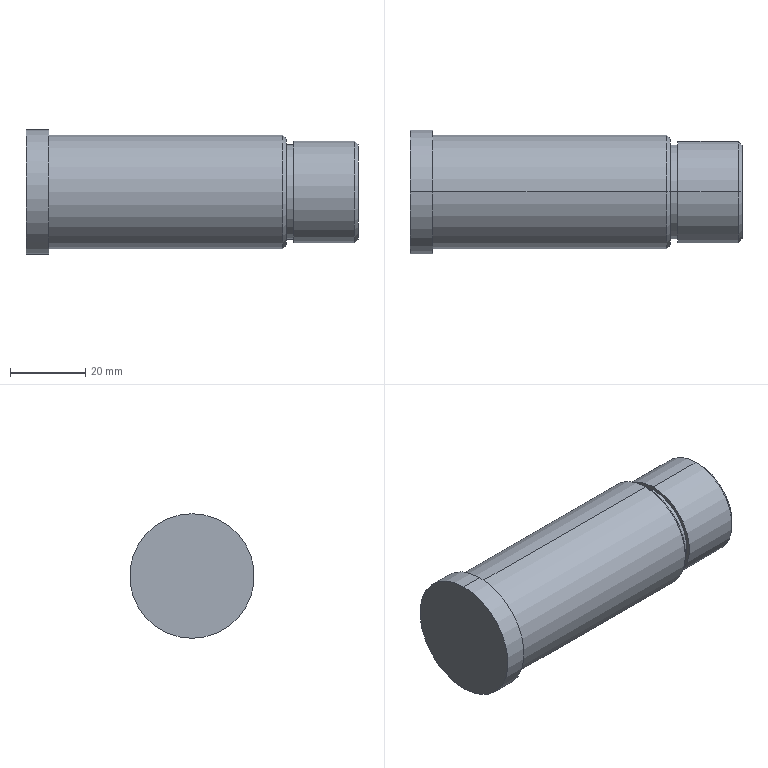Part | SolidWorks | features Chamfer 1, Revolution 1 | 1 solid | 17 faces | box 88 x 33 x 33 mm | volume 60292 mm3 | cylinder 8 | plane 5 | cone 4 | commonest cylinder face diameters 25 x2 27 x2 30 x2 33 x2
STEP:
#1=CARTESIAN_POINT('',(69.,0.,-14.));
#2=VERTEX_POINT('',#1);
#3=CARTESIAN_POINT('',(69.,0.,14.));
#4=VERTEX_POINT('',#3);
#5=CARTESIAN_POINT('',(69.,0.,0.));
#6=DIRECTION('',(1.,0.,0.));
#7=DIRECTION('',(0.,0.,1.));
#8=AXIS2_PLACEMENT_3D('',#5,#6,#7);
#9=CIRCLE('',#8,14.);
#10=EDGE_CURVE('',#2,#4,#9,.T.);
#11=ORIENTED_EDGE('',*,*,#10,.F.);
#12=CARTESIAN_POINT('',(68.,0.,-15.));
#13=VERTEX_POINT('',#12);
#14=CARTESIAN_POINT('',(68.,0.,-15.));
#15=DIRECTION('',(-0.7071,0.,-0.7071));
#16=VECTOR('',#15,1000.);
#17=LINE('',#14,#16);
#18=EDGE_CURVE('',#2,#13,#17,.T.);
#19=ORIENTED_EDGE('',*,*,#18,.T.);
#20=CARTESIAN_POINT('',(68.,0.,15.));
#21=VERTEX_POINT('',#20);
#22=CARTESIAN_POINT('',(68.,0.,0.));
#23=DIRECTION('',(-1.,0.,0.));
#24=DIRECTION('',(0.,0.,1.));
#25=AXIS2_PLACEMENT_3D('',#22,#23,#24);
#26=CIRCLE('',#25,15.);
#27=EDGE_CURVE('',#21,#13,#26,.T.);
#28=ORIENTED_EDGE('',*,*,#27,.F.);
#29=CARTESIAN_POINT('',(68.,0.,15.));
#30=DIRECTION('',(-0.7071,0.,0.7071));
#31=VECTOR('',#30,1000.);
#32=LINE('',#29,#31);
#33=EDGE_CURVE('',#4,#21,#32,.T.);
#34=ORIENTED_EDGE('',*,*,#33,.F.);
#35=EDGE_LOOP('',(#11,#19,#28,#34));
#36=FACE_OUTER_BOUND('',#35,.T.);
#37=CARTESIAN_POINT('',(68.,0.,0.));
#38=DIRECTION('',(-1.,0.,0.));
#39=DIRECTION('',(0.,0.,1.));
#40=AXIS2_PLACEMENT_3D('',#37,#38,#39);
#41=CONICAL_SURFACE('',#40,15.,0.7854);
#42=ADVANCED_FACE('',(#36),#41,.T.);
#43=CARTESIAN_POINT('',(88.,0.,-12.5));
#44=VERTEX_POINT('',#43);
#45=CARTESIAN_POINT('',(88.,0.,12.5));
#46=VERTEX_POINT('',#45);
#47=CARTESIAN_POINT('',(88.,0.,0.));
#48=DIRECTION('',(1.,0.,0.));
#49=DIRECTION('',(0.,0.,1.));
#50=AXIS2_PLACEMENT_3D('',#47,#48,#49);
#51=CIRCLE('',#50,12.5);
#52=EDGE_CURVE('',#44,#46,#51,.T.);
#53=ORIENTED_EDGE('',*,*,#52,.F.);
#54=CARTESIAN_POINT('',(87.,0.,-13.5));
#55=VERTEX_POINT('',#54);
#56=CARTESIAN_POINT('',(87.,0.,-13.5));
#57=DIRECTION('',(-0.7071,0.,-0.7071));
#58=VECTOR('',#57,1000.);
#59=LINE('',#56,#58);
#60=EDGE_CURVE('',#44,#55,#59,.T.);
#61=ORIENTED_EDGE('',*,*,#60,.T.);
#62=CARTESIAN_POINT('',(87.,0.,13.5));
#63=VERTEX_POINT('',#62);
#64=CARTESIAN_POINT('',(87.,0.,0.));
#65=DIRECTION('',(-1.,0.,0.));
#66=DIRECTION('',(0.,0.,1.));
#67=AXIS2_PLACEMENT_3D('',#64,#65,#66);
#68=CIRCLE('',#67,13.5);
#69=EDGE_CURVE('',#63,#55,#68,.T.);
#70=ORIENTED_EDGE('',*,*,#69,.F.);
#71=CARTESIAN_POINT('',(87.,0.,13.5));
#72=DIRECTION('',(-0.7071,0.,0.7071));
#73=VECTOR('',#72,1000.);
#74=LINE('',#71,#73);
#75=EDGE_CURVE('',#46,#63,#74,.T.);
#76=ORIENTED_EDGE('',*,*,#75,.F.);
#77=EDGE_LOOP('',(#53,#61,#70,#76));
#78=FACE_OUTER_BOUND('',#77,.T.);
#79=CARTESIAN_POINT('',(87.,0.,0.));
#80=DIRECTION('',(-1.,0.,0.));
#81=DIRECTION('',(0.,0.,1.));
#82=AXIS2_PLACEMENT_3D('',#79,#80,#81);
#83=CONICAL_SURFACE('',#82,13.5,0.7854);
#84=ADVANCED_FACE('',(#78),#83,.T.);
#85=ORIENTED_EDGE('',*,*,#69,.T.);
#86=CARTESIAN_POINT('',(71.,0.,-13.5));
#87=VERTEX_POINT('',#86);
#88=CARTESIAN_POINT('',(0.,0.,-13.5));
#89=DIRECTION('',(-1.,0.,0.));
#90=VECTOR('',#89,1000.);
#91=LINE('',#88,#90);
#92=EDGE_CURVE('',#55,#87,#91,.T.);
#93=ORIENTED_EDGE('',*,*,#92,.T.);
#94=CARTESIAN_POINT('',(71.,0.,13.5));
#95=VERTEX_POINT('',#94);
#96=CARTESIAN_POINT('',(71.,0.,0.));
#97=DIRECTION('',(-1.,0.,0.));
#98=DIRECTION('',(0.,0.,1.));
#99=AXIS2_PLACEMENT_3D('',#96,#97,#98);
#100=CIRCLE('',#99,13.5);
#101=EDGE_CURVE('',#95,#87,#100,.T.);
#102=ORIENTED_EDGE('',*,*,#101,.F.);
#103=CARTESIAN_POINT('',(0.,0.,13.5));
#104=DIRECTION('',(-1.,0.,0.));
#105=VECTOR('',#104,1000.);
#106=LINE('',#103,#105);
#107=EDGE_CURVE('',#63,#95,#106,.T.);
#108=ORIENTED_EDGE('',*,*,#107,.F.);
#109=EDGE_LOOP('',(#85,#93,#102,#108));
#110=FACE_OUTER_BOUND('',#109,.T.);
#111=CARTESIAN_POINT('',(0.,0.,0.));
#112=DIRECTION('',(-1.,0.,0.));
#113=DIRECTION('',(0.,0.,1.));
#114=AXIS2_PLACEMENT_3D('',#111,#112,#113);
#115=CYLINDRICAL_SURFACE('',#114,13.5);
#116=ADVANCED_FACE('',(#110),#115,.T.);
#117=CARTESIAN_POINT('',(71.,0.,12.5));
#118=VERTEX_POINT('',#117);
#119=CARTESIAN_POINT('',(71.,0.,-12.5));
#120=VERTEX_POINT('',#119);
#121=CARTESIAN_POINT('',(71.,0.,0.));
#122=DIRECTION('',(-1.,0.,0.));
#123=DIRECTION('',(0.,0.,1.));
#124=AXIS2_PLACEMENT_3D('',#121,#122,#123);
#125=CIRCLE('',#124,12.5);
#126=EDGE_CURVE('',#118,#120,#125,.T.);
#127=ORIENTED_EDGE('',*,*,#126,.T.);
#128=CARTESIAN_POINT('',(69.,0.,-12.5));
#129=VERTEX_POINT('',#128);
#130=CARTESIAN_POINT('',(0.,0.,-12.5));
#131=DIRECTION('',(-1.,0.,0.));
#132=VECTOR('',#131,1000.);
#133=LINE('',#130,#132);
#134=EDGE_CURVE('',#120,#129,#133,.T.);
#135=ORIENTED_EDGE('',*,*,#134,.T.);
#136=CARTESIAN_POINT('',(69.,0.,12.5));
#137=VERTEX_POINT('',#136);
#138=CARTESIAN_POINT('',(69.,0.,0.));
#139=DIRECTION('',(-1.,0.,0.));
#140=DIRECTION('',(0.,0.,1.));
#141=AXIS2_PLACEMENT_3D('',#138,#139,#140);
#142=CIRCLE('',#141,12.5);
#143=EDGE_CURVE('',#137,#129,#142,.T.);
#144=ORIENTED_EDGE('',*,*,#143,.F.);
#145=CARTESIAN_POINT('',(0.,0.,12.5));
#146=DIRECTION('',(-1.,0.,0.));
#147=VECTOR('',#146,1000.);
#148=LINE('',#145,#147);
#149=EDGE_CURVE('',#118,#137,#148,.T.);
#150=ORIENTED_EDGE('',*,*,#149,.F.);
#151=EDGE_LOOP('',(#127,#135,#144,#150));
#152=FACE_OUTER_BOUND('',#151,.T.);
#153=CARTESIAN_POINT('',(0.,0.,0.));
#154=DIRECTION('',(-1.,0.,0.));
#155=DIRECTION('',(0.,0.,1.));
#156=AXIS2_PLACEMENT_3D('',#153,#154,#155);
#157=CYLINDRICAL_SURFACE('',#156,12.5);
#158=ADVANCED_FACE('',(#152),#157,.T.);
#159=ORIENTED_EDGE('',*,*,#27,.T.);
#160=CARTESIAN_POINT('',(6.,0.,-15.));
#161=VERTEX_POINT('',#160);
#162=CARTESIAN_POINT('',(0.,0.,-15.));
#163=DIRECTION('',(-1.,0.,0.));
#164=VECTOR('',#163,1000.);
#165=LINE('',#162,#164);
#166=EDGE_CURVE('',#13,#161,#165,.T.);
#167=ORIENTED_EDGE('',*,*,#166,.T.);
#168=CARTESIAN_POINT('',(6.,0.,15.));
#169=VERTEX_POINT('',#168);
#170=CARTESIAN_POINT('',(6.,0.,0.));
#171=DIRECTION('',(-1.,0.,0.));
#172=DIRECTION('',(0.,0.,1.));
#173=AXIS2_PLACEMENT_3D('',#170,#171,#172);
#174=CIRCLE('',#173,15.);
#175=EDGE_CURVE('',#169,#161,#174,.T.);
#176=ORIENTED_EDGE('',*,*,#175,.F.);
#177=CARTESIAN_POINT('',(0.,0.,15.));
#178=DIRECTION('',(-1.,0.,0.));
#179=VECTOR('',#178,1000.);
#180=LINE('',#177,#179);
#181=EDGE_CURVE('',#21,#169,#180,.T.);
#182=ORIENTED_EDGE('',*,*,#181,.F.);
#183=EDGE_LOOP('',(#159,#167,#176,#182));
#184=FACE_OUTER_BOUND('',#183,.T.);
#185=CARTESIAN_POINT('',(0.,0.,0.));
#186=DIRECTION('',(-1.,0.,0.));
#187=DIRECTION('',(0.,0.,1.));
#188=AXIS2_PLACEMENT_3D('',#185,#186,#187);
#189=CYLINDRICAL_SURFACE('',#188,15.);
#190=ADVANCED_FACE('',(#184),#189,.T.);
#191=CARTESIAN_POINT('',(6.,0.,16.5));
#192=VERTEX_POINT('',#191);
#193=CARTESIAN_POINT('',(6.,0.,-16.5));
#194=VERTEX_POINT('',#193);
#195=CARTESIAN_POINT('',(6.,0.,0.));
#196=DIRECTION('',(-1.,0.,0.));
#197=DIRECTION('',(0.,0.,1.));
#198=AXIS2_PLACEMENT_3D('',#195,#196,#197);
#199=CIRCLE('',#198,16.5);
#200=EDGE_CURVE('',#192,#194,#199,.T.);
#201=ORIENTED_EDGE('',*,*,#200,.T.);
#202=CARTESIAN_POINT('',(0.,0.,-16.5));
#203=VERTEX_POINT('',#202);
#204=CARTESIAN_POINT('',(0.,0.,-16.5));
#205=DIRECTION('',(-1.,0.,0.));
#206=VECTOR('',#205,1000.);
#207=LINE('',#204,#206);
#208=EDGE_CURVE('',#194,#203,#207,.T.);
#209=ORIENTED_EDGE('',*,*,#208,.T.);
#210=CARTESIAN_POINT('',(0.,0.,16.5));
#211=VERTEX_POINT('',#210);
#212=CARTESIAN_POINT('',(0.,0.,0.));
#213=DIRECTION('',(-1.,0.,0.));
#214=DIRECTION('',(0.,0.,1.));
#215=AXIS2_PLACEMENT_3D('',#212,#213,#214);
#216=CIRCLE('',#215,16.5);
#217=EDGE_CURVE('',#211,#203,#216,.T.);
#218=ORIENTED_EDGE('',*,*,#217,.F.);
#219=CARTESIAN_POINT('',(0.,0.,16.5));
#220=DIRECTION('',(-1.,0.,0.));
#221=VECTOR('',#220,1000.);
#222=LINE('',#219,#221);
#223=EDGE_CURVE('',#192,#211,#222,.T.);
#224=ORIENTED_EDGE('',*,*,#223,.F.);
#225=EDGE_LOOP('',(#201,#209,#218,#224));
#226=FACE_OUTER_BOUND('',#225,.T.);
#227=CARTESIAN_POINT('',(0.,0.,0.));
#228=DIRECTION('',(-1.,0.,0.));
#229=DIRECTION('',(0.,0.,1.));
#230=AXIS2_PLACEMENT_3D('',#227,#228,#229);
#231=CYLINDRICAL_SURFACE('',#230,16.5);
#232=ADVANCED_FACE('',(#226),#231,.T.);
#233=ORIENTED_EDGE('',*,*,#217,.T.);
#234=CARTESIAN_POINT('',(0.,0.,0.));
#235=DIRECTION('',(-1.,0.,0.));
#236=DIRECTION('',(0.,0.,1.));
#237=AXIS2_PLACEMENT_3D('',#234,#235,#236);
#238=CIRCLE('',#237,16.5);
#239=EDGE_CURVE('',#203,#211,#238,.T.);
#240=ORIENTED_EDGE('',*,*,#239,.T.);
#241=EDGE_LOOP('',(#233,#240));
#242=FACE_OUTER_BOUND('',#241,.T.);
#243=CARTESIAN_POINT('',(0.,0.,0.));
#244=DIRECTION('',(1.,0.,0.));
#245=DIRECTION('',(0.,0.,-1.));
#246=AXIS2_PLACEMENT_3D('',#243,#244,#245);
#247=PLANE('',#246);
#248=ADVANCED_FACE('',(#242),#247,.F.);
#249=ORIENTED_EDGE('',*,*,#208,.F.);
#250=CARTESIAN_POINT('',(6.,0.,0.));
#251=DIRECTION('',(-1.,0.,0.));
#252=DIRECTION('',(0.,0.,1.));
#253=AXIS2_PLACEMENT_3D('',#250,#251,#252);
#254=CIRCLE('',#253,16.5);
#255=EDGE_CURVE('',#194,#192,#254,.T.);
#256=ORIENTED_EDGE('',*,*,#255,.T.);
#257=ORIENTED_EDGE('',*,*,#223,.T.);
#258=ORIENTED_EDGE('',*,*,#239,.F.);
#259=EDGE_LOOP('',(#249,#256,#257,#258));
#260=FACE_OUTER_BOUND('',#259,.T.);
#261=CARTESIAN_POINT('',(0.,0.,0.));
#262=DIRECTION('',(-1.,0.,0.));
#263=DIRECTION('',(0.,0.,1.));
#264=AXIS2_PLACEMENT_3D('',#261,#262,#263);
#265=CYLINDRICAL_SURFACE('',#264,16.5);
#266=ADVANCED_FACE('',(#260),#265,.T.);
#267=ORIENTED_EDGE('',*,*,#200,.F.);
#268=ORIENTED_EDGE('',*,*,#255,.F.);
#269=EDGE_LOOP('',(#267,#268));
#270=FACE_OUTER_BOUND('',#269,.T.);
#271=ORIENTED_EDGE('',*,*,#175,.T.);
#272=CARTESIAN_POINT('',(6.,0.,0.));
#273=DIRECTION('',(-1.,0.,0.));
#274=DIRECTION('',(0.,0.,1.));
#275=AXIS2_PLACEMENT_3D('',#272,#273,#274);
#276=CIRCLE('',#275,15.);
#277=EDGE_CURVE('',#161,#169,#276,.T.);
#278=ORIENTED_EDGE('',*,*,#277,.T.);
#279=EDGE_LOOP('',(#271,#278));
#280=FACE_BOUND('',#279,.T.);
#281=CARTESIAN_POINT('',(6.,16.5,0.));
#282=DIRECTION('',(-1.,0.,0.));
#283=DIRECTION('',(0.,0.,1.));
#284=AXIS2_PLACEMENT_3D('',#281,#282,#283);
#285=PLANE('',#284);
#286=ADVANCED_FACE('',(#270,#280),#285,.F.);
#287=ORIENTED_EDGE('',*,*,#166,.F.);
#288=CARTESIAN_POINT('',(68.,0.,0.));
#289=DIRECTION('',(-1.,0.,0.));
#290=DIRECTION('',(0.,0.,1.));
#291=AXIS2_PLACEMENT_3D('',#288,#289,#290);
#292=CIRCLE('',#291,15.);
#293=EDGE_CURVE('',#13,#21,#292,.T.);
#294=ORIENTED_EDGE('',*,*,#293,.T.);
#295=ORIENTED_EDGE('',*,*,#181,.T.);
#296=ORIENTED_EDGE('',*,*,#277,.F.);
#297=EDGE_LOOP('',(#287,#294,#295,#296));
#298=FACE_OUTER_BOUND('',#297,.T.);
#299=CARTESIAN_POINT('',(0.,0.,0.));
#300=DIRECTION('',(-1.,0.,0.));
#301=DIRECTION('',(0.,0.,1.));
#302=AXIS2_PLACEMENT_3D('',#299,#300,#301);
#303=CYLINDRICAL_SURFACE('',#302,15.);
#304=ADVANCED_FACE('',(#298),#303,.T.);
#305=CARTESIAN_POINT('',(69.,0.,0.));
#306=DIRECTION('',(1.,0.,0.));
#307=DIRECTION('',(0.,0.,1.));
#308=AXIS2_PLACEMENT_3D('',#305,#306,#307);
#309=CIRCLE('',#308,14.);
#310=EDGE_CURVE('',#4,#2,#309,.T.);
#311=ORIENTED_EDGE('',*,*,#310,.T.);
#312=ORIENTED_EDGE('',*,*,#10,.T.);
#313=EDGE_LOOP('',(#311,#312));
#314=FACE_OUTER_BOUND('',#313,.T.);
#315=ORIENTED_EDGE('',*,*,#143,.T.);
#316=CARTESIAN_POINT('',(69.,0.,0.));
#317=DIRECTION('',(-1.,0.,0.));
#318=DIRECTION('',(0.,0.,1.));
#319=AXIS2_PLACEMENT_3D('',#316,#317,#318);
#320=CIRCLE('',#319,12.5);
#321=EDGE_CURVE('',#129,#137,#320,.T.);
#322=ORIENTED_EDGE('',*,*,#321,.T.);
#323=EDGE_LOOP('',(#315,#322));
#324=FACE_BOUND('',#323,.T.);
#325=CARTESIAN_POINT('',(69.,15.,0.));
#326=DIRECTION('',(-1.,0.,0.));
#327=DIRECTION('',(0.,0.,1.));
#328=AXIS2_PLACEMENT_3D('',#325,#326,#327);
#329=PLANE('',#328);
#330=ADVANCED_FACE('',(#314,#324),#329,.F.);
#331=ORIENTED_EDGE('',*,*,#134,.F.);
#332=CARTESIAN_POINT('',(71.,0.,0.));
#333=DIRECTION('',(-1.,0.,0.));
#334=DIRECTION('',(0.,0.,1.));
#335=AXIS2_PLACEMENT_3D('',#332,#333,#334);
#336=CIRCLE('',#335,12.5);
#337=EDGE_CURVE('',#120,#118,#336,.T.);
#338=ORIENTED_EDGE('',*,*,#337,.T.);
#339=ORIENTED_EDGE('',*,*,#149,.T.);
#340=ORIENTED_EDGE('',*,*,#321,.F.);
#341=EDGE_LOOP('',(#331,#338,#339,#340));
#342=FACE_OUTER_BOUND('',#341,.T.);
#343=CARTESIAN_POINT('',(0.,0.,0.));
#344=DIRECTION('',(-1.,0.,0.));
#345=DIRECTION('',(0.,0.,1.));
#346=AXIS2_PLACEMENT_3D('',#343,#344,#345);
#347=CYLINDRICAL_SURFACE('',#346,12.5);
#348=ADVANCED_FACE('',(#342),#347,.T.);
#349=ORIENTED_EDGE('',*,*,#126,.F.);
#350=ORIENTED_EDGE('',*,*,#337,.F.);
#351=EDGE_LOOP('',(#349,#350));
#352=FACE_BOUND('',#351,.T.);
#353=ORIENTED_EDGE('',*,*,#101,.T.);
#354=CARTESIAN_POINT('',(71.,0.,0.));
#355=DIRECTION('',(-1.,0.,0.));
#356=DIRECTION('',(0.,0.,1.));
#357=AXIS2_PLACEMENT_3D('',#354,#355,#356);
#358=CIRCLE('',#357,13.5);
#359=EDGE_CURVE('',#87,#95,#358,.T.);
#360=ORIENTED_EDGE('',*,*,#359,.T.);
#361=EDGE_LOOP('',(#353,#360));
#362=FACE_OUTER_BOUND('',#361,.T.);
#363=CARTESIAN_POINT('',(71.,12.5,0.));
#364=DIRECTION('',(1.,0.,0.));
#365=DIRECTION('',(0.,0.,-1.));
#366=AXIS2_PLACEMENT_3D('',#363,#364,#365);
#367=PLANE('',#366);
#368=ADVANCED_FACE('',(#352,#362),#367,.F.);
#369=ORIENTED_EDGE('',*,*,#92,.F.);
#370=CARTESIAN_POINT('',(87.,0.,0.));
#371=DIRECTION('',(-1.,0.,0.));
#372=DIRECTION('',(0.,0.,1.));
#373=AXIS2_PLACEMENT_3D('',#370,#371,#372);
#374=CIRCLE('',#373,13.5);
#375=EDGE_CURVE('',#55,#63,#374,.T.);
#376=ORIENTED_EDGE('',*,*,#375,.T.);
#377=ORIENTED_EDGE('',*,*,#107,.T.);
#378=ORIENTED_EDGE('',*,*,#359,.F.);
#379=EDGE_LOOP('',(#369,#376,#377,#378));
#380=FACE_OUTER_BOUND('',#379,.T.);
#381=CARTESIAN_POINT('',(0.,0.,0.));
#382=DIRECTION('',(-1.,0.,0.));
#383=DIRECTION('',(0.,0.,1.));
#384=AXIS2_PLACEMENT_3D('',#381,#382,#383);
#385=CYLINDRICAL_SURFACE('',#384,13.5);
#386=ADVANCED_FACE('',(#380),#385,.T.);
#387=CARTESIAN_POINT('',(88.,0.,0.));
#388=DIRECTION('',(1.,0.,0.));
#389=DIRECTION('',(0.,0.,1.));
#390=AXIS2_PLACEMENT_3D('',#387,#388,#389);
#391=CIRCLE('',#390,12.5);
#392=EDGE_CURVE('',#46,#44,#391,.T.);
#393=ORIENTED_EDGE('',*,*,#392,.T.);
#394=ORIENTED_EDGE('',*,*,#52,.T.);
#395=EDGE_LOOP('',(#393,#394));
#396=FACE_OUTER_BOUND('',#395,.T.);
#397=CARTESIAN_POINT('',(88.,13.5,0.));
#398=DIRECTION('',(-1.,0.,0.));
#399=DIRECTION('',(0.,0.,1.));
#400=AXIS2_PLACEMENT_3D('',#397,#398,#399);
#401=PLANE('',#400);
#402=ADVANCED_FACE('',(#396),#401,.F.);
#403=ORIENTED_EDGE('',*,*,#60,.F.);
#404=ORIENTED_EDGE('',*,*,#392,.F.);
#405=ORIENTED_EDGE('',*,*,#75,.T.);
#406=ORIENTED_EDGE('',*,*,#375,.F.);
#407=EDGE_LOOP('',(#403,#404,#405,#406));
#408=FACE_OUTER_BOUND('',#407,.T.);
#409=CARTESIAN_POINT('',(87.,0.,0.));
#410=DIRECTION('',(-1.,0.,0.));
#411=DIRECTION('',(0.,0.,1.));
#412=AXIS2_PLACEMENT_3D('',#409,#410,#411);
#413=CONICAL_SURFACE('',#412,13.5,0.7854);
#414=ADVANCED_FACE('',(#408),#413,.T.);
#415=ORIENTED_EDGE('',*,*,#18,.F.);
#416=ORIENTED_EDGE('',*,*,#310,.F.);
#417=ORIENTED_EDGE('',*,*,#33,.T.);
#418=ORIENTED_EDGE('',*,*,#293,.F.);
#419=EDGE_LOOP('',(#415,#416,#417,#418));
#420=FACE_OUTER_BOUND('',#419,.T.);
#421=CARTESIAN_POINT('',(68.,0.,0.));
#422=DIRECTION('',(-1.,0.,0.));
#423=DIRECTION('',(0.,0.,1.));
#424=AXIS2_PLACEMENT_3D('',#421,#422,#423);
#425=CONICAL_SURFACE('',#424,15.,0.7854);
#426=ADVANCED_FACE('',(#420),#425,.T.);
#427=CLOSED_SHELL('',(#42,#84,#116,#158,#190,#232,#248,#266,#286,#304,#330,#348,#368,#386,#402,#414,#426));
#428=MANIFOLD_SOLID_BREP('',#427);
#429=CARTESIAN_POINT('',(0.,0.,0.));
#430=DIRECTION('',(0.,0.,1.));
#431=DIRECTION('',(1.,0.,0.));
#432=AXIS2_PLACEMENT_3D('',#429,#430,#431);
#433=(LENGTH_UNIT()NAMED_UNIT(*)SI_UNIT(.MILLI.,.METRE.));
#434=UNCERTAINTY_MEASURE_WITH_UNIT(LENGTH_MEASURE(0.00001),#433,'','');
#435=(NAMED_UNIT(*)PLANE_ANGLE_UNIT()SI_UNIT($,.RADIAN.));
#436=(NAMED_UNIT(*)SI_UNIT($,.STERADIAN.)SOLID_ANGLE_UNIT());
#437=(GEOMETRIC_REPRESENTATION_CONTEXT(3)GLOBAL_UNCERTAINTY_ASSIGNED_CONTEXT((#434))GLOBAL_UNIT_ASSIGNED_CONTEXT((#433,#435,#436))REPRESENTATION_CONTEXT('',''));
#438=ADVANCED_BREP_SHAPE_REPRESENTATION('',(#428,#432),#437);